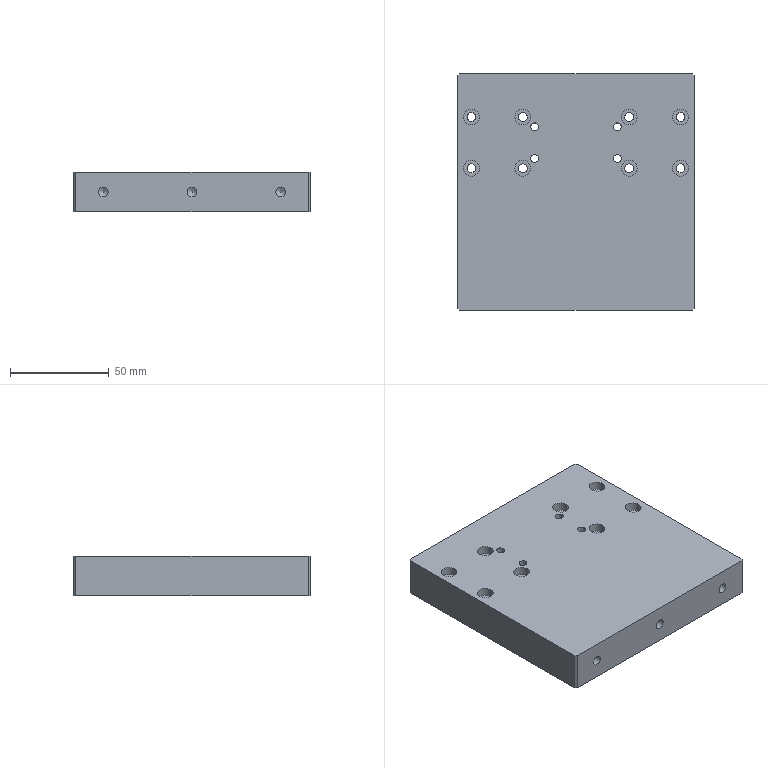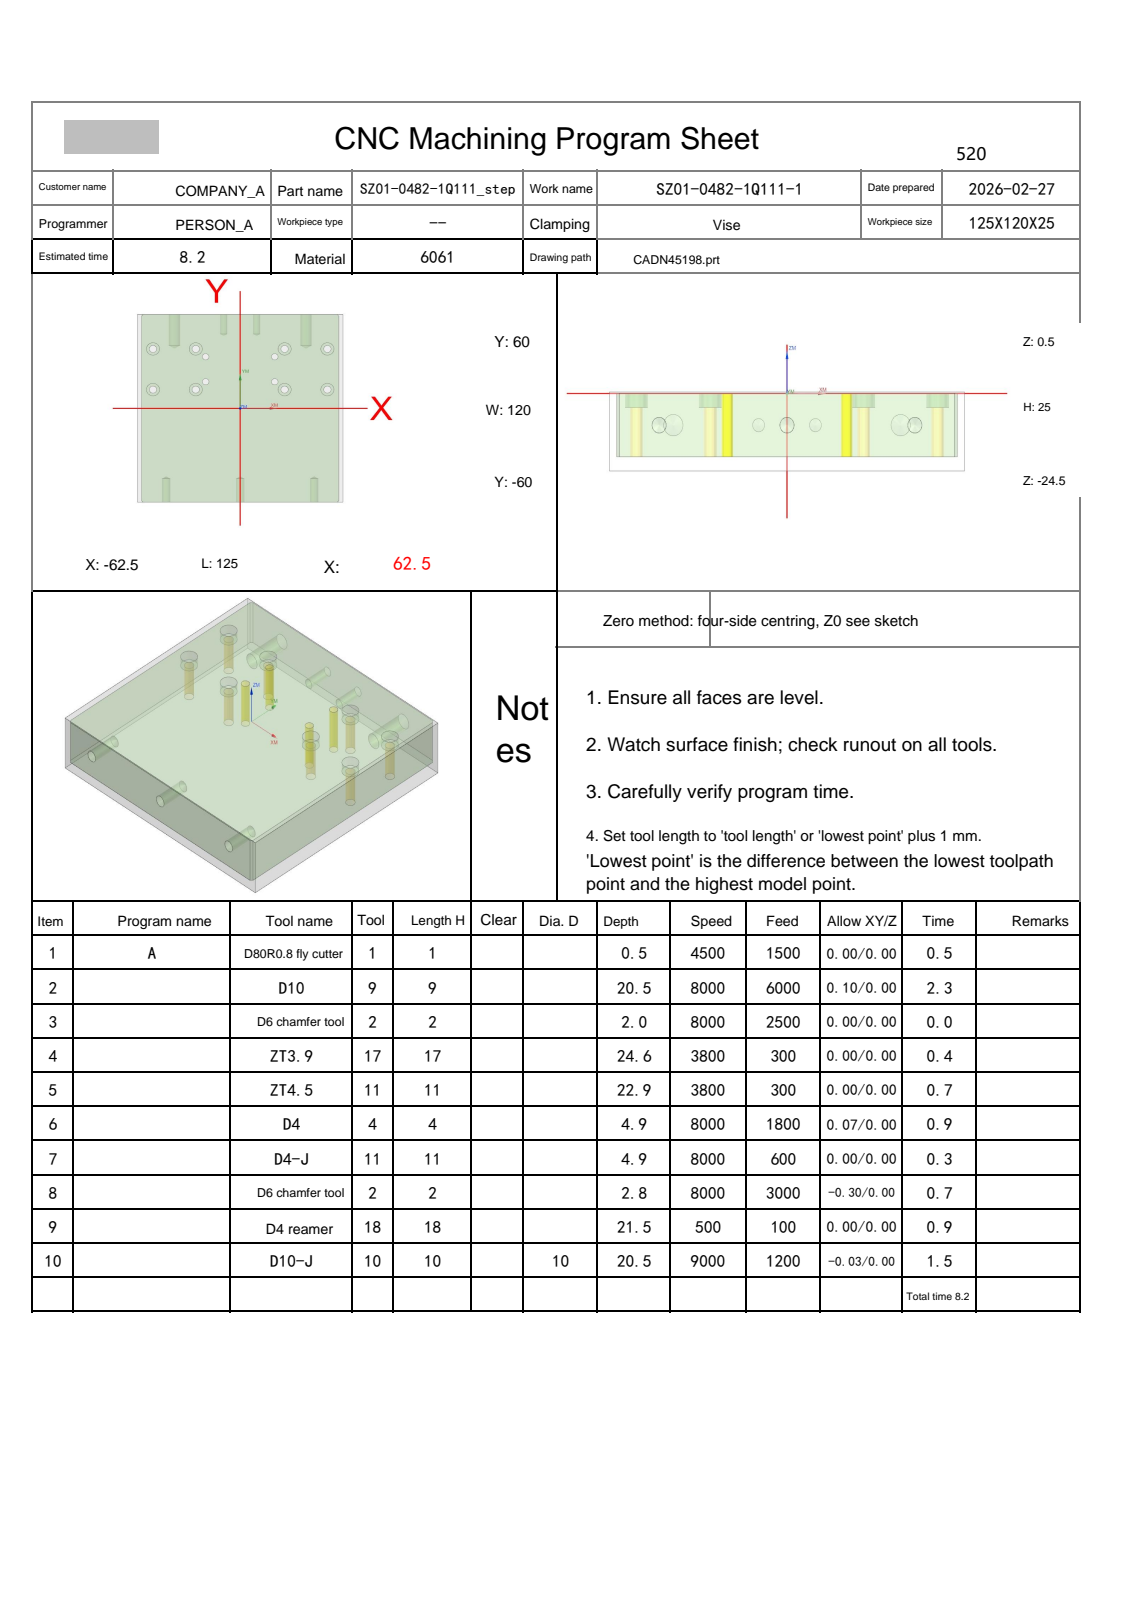NC program | NX | posted by the shop | part box 120 x 120 x 20 mm
Whole program:
%
O0001
(Machine time: 10.07 MIN)
(===Total Tool:8===)
(T1=D80R0.8 fly cutter D=80.  R=0.8  D-  H01 Z=0.    )
(T9=D10     D=10.  R=0.   D-  H09 Z=-20.  )
(T2=D6 chamfer tool   D=6.   R=0.   D-  H02 Z=-2.3  )
(T17=ZT3.9  D=3.9  DR_a=120 D-  H17 Z=-24.13)
(T11=ZT4.5  D=4.5  DR_a=118 D-  H11 Z=-22.35)
(T4=D4      D=4.   R=0.   D-  H04 Z=-4.4  )
(T18=D4 reamer   D=4.   DR_a=180 D-  H18 Z=-21.  )
(T10=D10-J  D=10.  R=0.   D10 H10 Z=-20.  )
G80 G90 G17 G49 G40
G91 G28 Z0
M01
N1 T01 M06
(D80R0.8 fly cutter  D=80. R=0.8 H=01 ce=0.00 di=0.00)
G00 G90 G54 X-105. Y50. M03 S4500
G43 H01 Z50.
M08
Z2.
G01 Z0.0 F1500.
X-100.
X100.
Y0.0
X-100.
Y-50.
X100.
X105.
Z2.
G00 Z50.
G91 G28 Z0.0
M05
M09
G91 G28 Z0.0
M01
N2 T09 M06
(D10  D=10. R=0. H=09 ce=0.10 di=0.00)
G00 G90 G54 X65.1 Y0.0 M03 S8000
G43 H09 Z50.
M08
Z.5
G01 Y-59. Z.409 F6000.
G02 X63.606 Y-62.606 Z.403 I-5.1 J0.0
G01 X62.606 Y-63.606 Z.4
G02 X59. Y-65.1 Z.394 I-3.606 J3.606
G01 X-59. Z.212
G02 X-61.112 Y-64.642 Z.208 I0.0 J5.1
X-62.606 Y-63.606 Z.205 I2.112 J4.642
G01 X-63.606 Y-62.606 Z.203
G02 X-65.1 Y-59. Z.197 I3.606 J3.606
G01 Y59. Z.015
G02 X-63.606 Y62.606 Z.008 I5.1 J0.0
G01 X-62.606 Y63.606 Z.006
G02 X-59. Y65.1 Z0.0 I3.606 J-3.606
G01 X59. Z-.183
G02 X62.606 Y63.606 Z-.189 I0.0 J-5.1
G01 X63.606 Y62.606 Z-.191
G02 X65.1 Y59. Z-.197 I-3.606 J-3.606
G01 Y-59. Z-.38
G02 X63.606 Y-62.606 Z-.386 I-5.1 J0.0
G01 X62.606 Y-63.606 Z-.388
G02 X59. Y-65.1 Z-.394 I-3.606 J3.606
G01 X-59. Z-.577
G02 X-61.112 Y-64.642 Z-.58 I0.0 J5.1
X-62.606 Y-63.606 Z-.583 I2.112 J4.642
G01 X-63.606 Y-62.606 Z-.585
G02 X-65.1 Y-59. Z-.591 I3.606 J3.606
G01 Y59. Z-.774
G02 X-63.606 Y62.606 Z-.78 I5.1 J0.0
G01 X-62.606 Y63.606 Z-.782
G02 X-59. Y65.1 Z-.789 I3.606 J-3.606
G01 X59. Z-.971
G02 X62.606 Y63.606 Z-.977 I0.0 J-5.1
G01 X63.606 Y62.606 Z-.979
G02 X65.1 Y59. Z-.986 I-3.606 J-3.606
G01 Y-59. Z-1.168
G02 X63.606 Y-62.606 Z-1.174 I-5.1 J0.0
G01 X62.606 Y-63.606 Z-1.177
G02 X59. Y-65.1 Z-1.183 I-3.606 J3.606
G01 X-59. Z-1.365
G02 X-61.112 Y-64.642 Z-1.369 I0.0 J5.1
X-62.606 Y-63.606 Z-1.372 I2.112 J4.642
G01 X-63.606 Y-62.606 Z-1.374
G02 X-65.1 Y-59. Z-1.38 I3.606 J3.606
G01 Y59. Z-1.562
G02 X-63.606 Y62.606 Z-1.569 I5.1 J0.0
G01 X-62.606 Y63.606 Z-1.571
G02 X-59. Y65.1 Z-1.577 I3.606 J-3.606
G01 X59. Z-1.76
G02 X62.606 Y63.606 Z-1.766 I0.0 J-5.1
G01 X63.606 Y62.606 Z-1.768
G02 X65.1 Y59. Z-1.774 I-3.606 J-3.606
G01 Y-59. Z-1.957
G02 X63.606 Y-62.606 Z-1.963 I-5.1 J0.0
G01 X62.606 Y-63.606 Z-1.965
G02 X59. Y-65.1 Z-1.971 I-3.606 J3.606
G01 X-59. Z-2.154
G02 X-61.112 Y-64.642 Z-2.157 I0.0 J5.1
X-62.606 Y-63.606 Z-2.16 I2.112 J4.642
G01 X-63.606 Y-62.606 Z-2.162
G02 X-65.1 Y-59. Z-2.168 I3.606 J3.606
G01 Y59. Z-2.351
G02 X-63.606 Y62.606 Z-2.357 I5.1 J0.0
G01 X-62.606 Y63.606 Z-2.359
G02 X-59. Y65.1 Z-2.365 I3.606 J-3.606
G01 X59. Z-2.548
G02 X62.606 Y63.606 Z-2.554 I0.0 J-5.1
G01 X63.606 Y62.606 Z-2.556
G02 X65.1 Y59. Z-2.563 I-3.606 J-3.606
G01 Y-59. Z-2.745
G02 X63.606 Y-62.606 Z-2.751 I-5.1 J0.0
G01 X62.606 Y-63.606 Z-2.753
G02 X59. Y-65.1 Z-2.76 I-3.606 J3.606
G01 X-59. Z-2.942
G02 X-61.112 Y-64.642 Z-2.946 I0.0 J5.1
X-62.606 Y-63.606 Z-2.948 I2.112 J4.642
G01 X-63.606 Y-62.606 Z-2.951
G02 X-65.1 Y-59. Z-2.957 I3.606 J3.606
G01 Y59. Z-3.139
G02 X-63.606 Y62.606 Z-3.146 I5.1 J0.0
G01 X-62.606 Y63.606 Z-3.148
G02 X-59. Y65.1 Z-3.154 I3.606 J-3.606
G01 X59. Z-3.336
G02 X62.606 Y63.606 Z-3.343 I0.0 J-5.1
G01 X63.606 Y62.606 Z-3.345
G02 X65.1 Y59. Z-3.351 I-3.606 J-3.606
G01 Y-59. Z-3.534
G02 X63.606 Y-62.606 Z-3.54 I-5.1 J0.0
G01 X62.606 Y-63.606 Z-3.542
G02 X59. Y-65.1 Z-3.548 I-3.606 J3.606
G01 X-59. Z-3.731
G02 X-61.112 Y-64.642 Z-3.734 I0.0 J5.1
X-62.606 Y-63.606 Z-3.737 I2.112 J4.642
G01 X-63.606 Y-62.606 Z-3.739
G02 X-65.1 Y-59. Z-3.745 I3.606 J3.606
G01 Y59. Z-3.928
G02 X-63.606 Y62.606 Z-3.934 I5.1 J0.0
G01 X-62.606 Y63.606 Z-3.936
G02 X-59. Y65.1 Z-3.942 I3.606 J-3.606
G01 X59. Z-4.125
G02 X62.606 Y63.606 Z-4.131 I0.0 J-5.1
G01 X63.606 Y62.606 Z-4.133
G02 X65.1 Y59. Z-4.14 I-3.606 J-3.606
G01 Y-59. Z-4.322
G02 X63.606 Y-62.606 Z-4.328 I-5.1 J0.0
G01 X62.606 Y-63.606 Z-4.33
G02 X59. Y-65.1 Z-4.337 I-3.606 J3.606
G01 X-59. Z-4.519
G02 X-61.112 Y-64.642 Z-4.523 I0.0 J5.1
X-62.606 Y-63.606 Z-4.525 I2.112 J4.642
G01 X-63.606 Y-62.606 Z-4.528
G02 X-65.1 Y-59. Z-4.534 I3.606 J3.606
G01 Y59. Z-4.716
G02 X-63.606 Y62.606 Z-4.722 I5.1 J0.0
G01 X-62.606 Y63.606 Z-4.725
G02 X-59. Y65.1 Z-4.731 I3.606 J-3.606
G01 X59. Z-4.913
G02 X62.606 Y63.606 Z-4.92 I0.0 J-5.1
G01 X63.606 Y62.606 Z-4.922
G02 X65.1 Y59. Z-4.928 I-3.606 J-3.606
G01 Y-59. Z-5.11
G02 X63.606 Y-62.606 Z-5.117 I-5.1 J0.0
G01 X62.606 Y-63.606 Z-5.119
G02 X59. Y-65.1 Z-5.125 I-3.606 J3.606
G01 X-59. Z-5.308
G02 X-61.112 Y-64.642 Z-5.311 I0.0 J5.1
X-62.606 Y-63.606 Z-5.314 I2.112 J4.642
G01 X-63.606 Y-62.606 Z-5.316
G02 X-65.1 Y-59. Z-5.322 I3.606 J3.606
G01 Y59. Z-5.505
G02 X-63.606 Y62.606 Z-5.511 I5.1 J0.0
G01 X-62.606 Y63.606 Z-5.513
G02 X-59. Y65.1 Z-5.519 I3.606 J-3.606
G01 X59. Z-5.702
G02 X62.606 Y63.606 Z-5.708 I0.0 J-5.1
G01 X63.606 Y62.606 Z-5.71
G02 X65.1 Y59. Z-5.716 I-3.606 J-3.606
G01 Y-59. Z-5.899
G02 X63.606 Y-62.606 Z-5.905 I-5.1 J0.0
G01 X62.606 Y-63.606 Z-5.907
G02 X59. Y-65.1 Z-5.914 I-3.606 J3.606
G01 X-59. Z-6.096
G02 X-61.112 Y-64.642 Z-6.099 I0.0 J5.1
X-62.606 Y-63.606 Z-6.102 I2.112 J4.642
G01 X-63.606 Y-62.606 Z-6.104
G02 X-65.1 Y-59. Z-6.111 I3.606 J3.606
G01 Y59. Z-6.293
G02 X-63.606 Y62.606 Z-6.299 I5.1 J0.0
G01 X-62.606 Y63.606 Z-6.302
G02 X-59. Y65.1 Z-6.308 I3.606 J-3.606
G01 X59. Z-6.49
G02 X62.606 Y63.606 Z-6.497 I0.0 J-5.1
G01 X63.606 Y62.606 Z-6.499
G02 X65.1 Y59. Z-6.505 I-3.606 J-3.606
G01 Y-59. Z-6.687
G02 X63.606 Y-62.606 Z-6.694 I-5.1 J0.0
G01 X62.606 Y-63.606 Z-6.696
G02 X59. Y-65.1 Z-6.702 I-3.606 J3.606
G01 X-59. Z-6.885
G02 X-61.112 Y-64.642 Z-6.888 I0.0 J5.1
X-62.606 Y-63.606 Z-6.891 I2.112 J4.642
G01 X-63.606 Y-62.606 Z-6.893
G02 X-65.1 Y-59. Z-6.899 I3.606 J3.606
G01 Y59. Z-7.082
G02 X-63.606 Y62.606 Z-7.088 I5.1 J0.0
G01 X-62.606 Y63.606 Z-7.09
G02 X-59. Y65.1 Z-7.096 I3.606 J-3.606
G01 X59. Z-7.279
G02 X62.606 Y63.606 Z-7.285 I0.0 J-5.1
G01 X63.606 Y62.606 Z-7.287
G02 X65.1 Y59. Z-7.293 I-3.606 J-3.606
G01 Y-59. Z-7.476
G02 X63.606 Y-62.606 Z-7.482 I-5.1 J0.0
G01 X62.606 Y-63.606 Z-7.484
G02 X59. Y-65.1 Z-7.49 I-3.606 J3.606
G01 X-59. Z-7.673
G02 X-61.112 Y-64.642 Z-7.676 I0.0 J5.1
X-62.606 Y-63.606 Z-7.679 I2.112 J4.642
G01 X-63.606 Y-62.606 Z-7.681
G02 X-65.1 Y-59. Z-7.688 I3.606 J3.606
G01 Y59. Z-7.87
G02 X-63.606 Y62.606 Z-7.876 I5.1 J0.0
G01 X-62.606 Y63.606 Z-7.878
G02 X-59. Y65.1 Z-7.885 I3.606 J-3.606
G01 X59. Z-8.067
G02 X62.606 Y63.606 Z-8.073 I0.0 J-5.1
G01 X63.606 Y62.606 Z-8.076
G02 X65.1 Y59. Z-8.082 I-3.606 J-3.606
G01 Y-59. Z-8.264
G02 X63.606 Y-62.606 Z-8.271 I-5.1 J0.0
G01 X62.606 Y-63.606 Z-8.273
G02 X59. Y-65.1 Z-8.279 I-3.606 J3.606
G01 X-59. Z-8.461
G02 X-61.112 Y-64.642 Z-8.465 I0.0 J5.1
X-62.606 Y-63.606 Z-8.468 I2.112 J4.642
G01 X-63.606 Y-62.606 Z-8.47
G02 X-65.1 Y-59. Z-8.476 I3.606 J3.606
G01 Y59. Z-8.659
G02 X-63.606 Y62.606 Z-8.665 I5.1 J0.0
G01 X-62.606 Y63.606 Z-8.667
G02 X-59. Y65.1 Z-8.673 I3.606 J-3.606
G01 X59. Z-8.856
G02 X62.606 Y63.606 Z-8.862 I0.0 J-5.1
G01 X63.606 Y62.606 Z-8.864
G02 X65.1 Y59. Z-8.87 I-3.606 J-3.606
G01 Y-59. Z-9.053
G02 X63.606 Y-62.606 Z-9.059 I-5.1 J0.0
G01 X62.606 Y-63.606 Z-9.061
G02 X59. Y-65.1 Z-9.067 I-3.606 J3.606
G01 X-59. Z-9.25
G02 X-61.112 Y-64.642 Z-9.253 I0.0 J5.1
X-62.606 Y-63.606 Z-9.256 I2.112 J4.642
G01 X-63.606 Y-62.606 Z-9.258
G02 X-65.1 Y-59. Z-9.265 I3.606 J3.606
G01 Y59. Z-9.447
G02 X-63.606 Y62.606 Z-9.453 I5.1 J0.0
G01 X-62.606 Y63.606 Z-9.455
G02 X-59. Y65.1 Z-9.462 I3.606 J-3.606
G01 X59. Z-9.644
G02 X62.606 Y63.606 Z-9.65 I0.0 J-5.1
G01 X63.606 Y62.606 Z-9.653
G02 X65.1 Y59. Z-9.659 I-3.606 J-3.606
G01 Y-59. Z-9.841
G02 X63.606 Y-62.606 Z-9.847 I-5.1 J0.0
G01 X62.606 Y-63.606 Z-9.85
G02 X59. Y-65.1 Z-9.856 I-3.606 J3.606
G01 X-59. Z-10.038
G02 X-61.112 Y-64.642 Z-10.042 I0.0 J5.1
X-62.606 Y-63.606 Z-10.045 I2.112 J4.642
G01 X-63.606 Y-62.606 Z-10.047
G02 X-65.1 Y-59. Z-10.053 I3.606 J3.606
G01 Y59. Z-10.235
G02 X-63.606 Y62.606 Z-10.242 I5.1 J0.0
G01 X-62.606 Y63.606 Z-10.244
G02 X-59. Y65.1 Z-10.25 I3.606 J-3.606
G01 X59. Z-10.433
G02 X62.606 Y63.606 Z-10.439 I0.0 J-5.1
G01 X63.606 Y62.606 Z-10.441
G02 X65.1 Y59. Z-10.447 I-3.606 J-3.606
G01 Y-59. Z-10.63
G02 X63.606 Y-62.606 Z-10.636 I-5.1 J0.0
G01 X62.606 Y-63.606 Z-10.638
G02 X59. Y-65.1 Z-10.644 I-3.606 J3.606
G01 X-59. Z-10.827
G02 X-61.112 Y-64.642 Z-10.83 I0.0 J5.1
X-62.606 Y-63.606 Z-10.833 I2.112 J4.642
G01 X-63.606 Y-62.606 Z-10.835
G02 X-65.1 Y-59. Z-10.841 I3.606 J3.606
G01 Y59. Z-11.024
G02 X-63.606 Y62.606 Z-11.03 I5.1 J0.0
G01 X-62.606 Y63.606 Z-11.032
G02 X-59. Y65.1 Z-11.039 I3.606 J-3.606
G01 X59. Z-11.221
G02 X62.606 Y63.606 Z-11.227 I0.0 J-5.1
G01 X63.606 Y62.606 Z-11.229
G02 X65.1 Y59. Z-11.236 I-3.606 J-3.606
G01 Y-59. Z-11.418
G02 X63.606 Y-62.606 Z-11.424 I-5.1 J0.0
G01 X62.606 Y-63.606 Z-11.427
G02 X59. Y-65.1 Z-11.433 I-3.606 J3.606
G01 X-59. Z-11.615
G02 X-61.112 Y-64.642 Z-11.619 I0.0 J5.1
X-62.606 Y-63.606 Z-11.622 I2.112 J4.642
G01 X-63.606 Y-62.606 Z-11.624
G02 X-65.1 Y-59. Z-11.63 I3.606 J3.606
G01 Y59. Z-11.812
G02 X-63.606 Y62.606 Z-11.819 I5.1 J0.0
G01 X-62.606 Y63.606 Z-11.821
G02 X-59. Y65.1 Z-11.827 I3.606 J-3.606
G01 X59. Z-12.01
G02 X62.606 Y63.606 Z-12.016 I0.0 J-5.1
G01 X63.606 Y62.606 Z-12.018
G02 X65.1 Y59. Z-12.024 I-3.606 J-3.606
G01 Y-59. Z-12.207
G02 X63.606 Y-62.606 Z-12.213 I-5.1 J0.0
G01 X62.606 Y-63.606 Z-12.215
G02 X59. Y-65.1 Z-12.221 I-3.606 J3.606
G01 X-59. Z-12.404
G02 X-61.112 Y-64.642 Z-12.407 I0.0 J5.1
X-62.606 Y-63.606 Z-12.41 I2.112 J4.642
G01 X-63.606 Y-62.606 Z-12.412
G02 X-65.1 Y-59. Z-12.418 I3.606 J3.606
G01 Y59. Z-12.601
G02 X-63.606 Y62.606 Z-12.607 I5.1 J0.0
G01 X-62.606 Y63.606 Z-12.609
G02 X-59. Y65.1 Z-12.615 I3.606 J-3.606
G01 X59. Z-12.798
G02 X62.606 Y63.606 Z-12.804 I0.0 J-5.1
G01 X63.606 Y62.606 Z-12.806
G02 X65.1 Y59. Z-12.813 I-3.606 J-3.606
G01 Y-59. Z-12.995
G02 X63.606 Y-62.606 Z-13.001 I-5.1 J0.0
G01 X62.606 Y-63.606 Z-13.003
G02 X59. Y-65.1 Z-13.01 I-3.606 J3.606
G01 X-59. Z-13.192
G02 X-61.112 Y-64.642 Z-13.196 I0.0 J5.1
X-62.606 Y-63.606 Z-13.198 I2.112 J4.642
G01 X-63.606 Y-62.606 Z-13.201
G02 X-65.1 Y-59. Z-13.207 I3.606 J3.606
G01 Y59. Z-13.389
G02 X-63.606 Y62.606 Z-13.396 I5.1 J0.0
G01 X-62.606 Y63.606 Z-13.398
G02 X-59. Y65.1 Z-13.404 I3.606 J-3.606
G01 X59. Z-13.586
G02 X62.606 Y63.606 Z-13.593 I0.0 J-5.1
G01 X63.606 Y62.606 Z-13.595
G02 X65.1 Y59. Z-13.601 I-3.606 J-3.606
G01 Y-59. Z-13.784
G02 X63.606 Y-62.606 Z-13.79 I-5.1 J0.0
G01 X62.606 Y-63.606 Z-13.792
G02 X59. Y-65.1 Z-13.798 I-3.606 J3.606
G01 X-59. Z-13.981
G02 X-61.112 Y-64.642 Z-13.984 I0.0 J5.1
X-62.606 Y-63.606 Z-13.987 I2.112 J4.642
G01 X-63.606 Y-62.606 Z-13.989
G02 X-65.1 Y-59. Z-13.995 I3.606 J3.606
G01 Y59. Z-14.178
G02 X-63.606 Y62.606 Z-14.184 I5.1 J0.0
G01 X-62.606 Y63.606 Z-14.186
G02 X-59. Y65.1 Z-14.192 I3.606 J-3.606
G01 X59. Z-14.375
G02 X62.606 Y63.606 Z-14.381 I0.0 J-5.1
G01 X63.606 Y62.606 Z-14.383
G02 X65.1 Y59. Z-14.39 I-3.606 J-3.606
G01 Y-59. Z-14.572
G02 X63.606 Y-62.606 Z-14.578 I-5.1 J0.0
G01 X62.606 Y-63.606 Z-14.58
G02 X59. Y-65.1 Z-14.587 I-3.606 J3.606
G01 X-59. Z-14.769
G02 X-61.112 Y-64.642 Z-14.773 I0.0 J5.1
X-62.606 Y-63.606 Z-14.775 I2.112 J4.642
G01 X-63.606 Y-62.606 Z-14.778
G02 X-65.1 Y-59. Z-14.784 I3.606 J3.606
G01 Y59. Z-14.966
G02 X-63.606 Y62.606 Z-14.972 I5.1 J0.0
G01 X-62.606 Y63.606 Z-14.975
G02 X-59. Y65.1 Z-14.981 I3.606 J-3.606
G01 X59. Z-15.163
G02 X62.606 Y63.606 Z-15.17 I0.0 J-5.1
G01 X63.606 Y62.606 Z-15.172
G02 X65.1 Y59. Z-15.178 I-3.606 J-3.606
G01 Y-59. Z-15.36
G02 X63.606 Y-62.606 Z-15.367 I-5.1 J0.0
G01 X62.606 Y-63.606 Z-15.369
G02 X59. Y-65.1 Z-15.375 I-3.606 J3.606
G01 X-59. Z-15.558
G02 X-61.112 Y-64.642 Z-15.561 I0.0 J5.1
X-62.606 Y-63.606 Z-15.564 I2.112 J4.642
G01 X-63.606 Y-62.606 Z-15.566
G02 X-65.1 Y-59. Z-15.572 I3.606 J3.606
G01 Y59. Z-15.755
G02 X-63.606 Y62.606 Z-15.761 I5.1 J0.0
G01 X-62.606 Y63.606 Z-15.763
G02 X-59. Y65.1 Z-15.769 I3.606 J-3.606
G01 X59. Z-15.952
G02 X62.606 Y63.606 Z-15.958 I0.0 J-5.1
G01 X63.606 Y62.606 Z-15.96
G02 X65.1 Y59. Z-15.966 I-3.606 J-3.606
G01 Y-59. Z-16.149
G02 X63.606 Y-62.606 Z-16.155 I-5.1 J0.0
G01 X62.606 Y-63.606 Z-16.157
G02 X59. Y-65.1 Z-16.164 I-3.606 J3.606
G01 X-59. Z-16.346
G02 X-61.112 Y-64.642 Z-16.349 I0.0 J5.1
X-62.606 Y-63.606 Z-16.352 I2.112 J4.642
G01 X-63.606 Y-62.606 Z-16.354
G02 X-65.1 Y-59. Z-16.361 I3.606 J3.606
G01 Y59. Z-16.543
G02 X-63.606 Y62.606 Z-16.549 I5.1 J0.0
G01 X-62.606 Y63.606 Z-16.552
G02 X-59. Y65.1 Z-16.558 I3.606 J-3.606
G01 X59. Z-16.74
G02 X62.606 Y63.606 Z-16.747 I0.0 J-5.1
G01 X63.606 Y62.606 Z-16.749
G02 X65.1 Y59. Z-16.755 I-3.606 J-3.606
G01 Y-59. Z-16.937
G02 X63.606 Y-62.606 Z-16.944 I-5.1 J0.0
G01 X62.606 Y-63.606 Z-16.946
G02 X59. Y-65.1 Z-16.952 I-3.606 J3.606
G01 X-59. Z-17.135
G02 X-61.112 Y-64.642 Z-17.138 I0.0 J5.1
X-62.606 Y-63.606 Z-17.141 I2.112 J4.642
G01 X-63.606 Y-62.606 Z-17.143
G02 X-65.1 Y-59. Z-17.149 I3.606 J3.606
G01 Y59. Z-17.332
G02 X-63.606 Y62.606 Z-17.338 I5.1 J0.0
G01 X-62.606 Y63.606 Z-17.34
G02 X-59. Y65.1 Z-17.346 I3.606 J-3.606
G01 X59. Z-17.529
G02 X62.606 Y63.606 Z-17.535 I0.0 J-5.1
G01 X63.606 Y62.606 Z-17.537
G02 X65.1 Y59. Z-17.543 I-3.606 J-3.606
G01 Y-59. Z-17.726
G02 X63.606 Y-62.606 Z-17.732 I-5.1 J0.0
G01 X62.606 Y-63.606 Z-17.734
G02 X59. Y-65.1 Z-17.74 I-3.606 J3.606
G01 X-59. Z-17.923
G02 X-61.112 Y-64.642 Z-17.926 I0.0 J5.1
X-62.606 Y-63.606 Z-17.929 I2.112 J4.642
G01 X-63.606 Y-62.606 Z-17.931
G02 X-65.1 Y-59. Z-17.938 I3.606 J3.606
G01 Y59. Z-18.12
G02 X-63.606 Y62.606 Z-18.126 I5.1 J0.0
G01 X-62.606 Y63.606 Z-18.128
G02 X-59. Y65.1 Z-18.135 I3.606 J-3.606
G01 X59. Z-18.317
G02 X62.606 Y63.606 Z-18.323 I0.0 J-5.1
G01 X63.606 Y62.606 Z-18.326
G02 X65.1 Y59. Z-18.332 I-3.606 J-3.606
G01 Y-59. Z-18.514
G02 X63.606 Y-62.606 Z-18.521 I-5.1 J0.0
G01 X62.606 Y-63.606 Z-18.523
G02 X59. Y-65.1 Z-18.529 I-3.606 J3.606
G01 X-59. Z-18.711
G02 X-61.112 Y-64.642 Z-18.715 I0.0 J5.1
X-62.606 Y-63.606 Z-18.718 I2.112 J4.642
G01 X-63.606 Y-62.606 Z-18.72
G02 X-65.1 Y-59. Z-18.726 I3.606 J3.606
G01 Y59. Z-18.909
G02 X-63.606 Y62.606 Z-18.915 I5.1 J0.0
G01 X-62.606 Y63.606 Z-18.917
G02 X-59. Y65.1 Z-18.923 I3.606 J-3.606
G01 X59. Z-19.106
G02 X62.606 Y63.606 Z-19.112 I0.0 J-5.1
G01 X63.606 Y62.606 Z-19.114
G02 X65.1 Y59. Z-19.12 I-3.606 J-3.606
G01 Y-59. Z-19.303
G02 X63.606 Y-62.606 Z-19.309 I-5.1 J0.0
G01 X62.606 Y-63.606 Z-19.311
G02 X59. Y-65.1 Z-19.317 I-3.606 J3.606
G01 X-59. Z-19.5
G02 X-61.112 Y-64.642 Z-19.503 I0.0 J5.1
X-62.606 Y-63.606 Z-19.506 I2.112 J4.642
G01 X-63.606 Y-62.606 Z-19.508
G02 X-65.1 Y-59. Z-19.515 I3.606 J3.606
G01 Y59. Z-19.697
G02 X-63.606 Y62.606 Z-19.703 I5.1 J0.0
G01 X-62.606 Y63.606 Z-19.705
G02 X-59. Y65.1 Z-19.712 I3.606 J-3.606
G01 X59. Z-19.894
G02 X62.606 Y63.606 Z-19.9 I0.0 J-5.1
G01 X63.606 Y62.606 Z-19.903
G02 X65.1 Y59. Z-19.909 I-3.606 J-3.606
G01 Y0.0 Z-20.
Y-59.
G02 X63.606 Y-62.606 I-5.1 J0.0
G01 X62.606 Y-63.606
G02 X59. Y-65.1 I-3.606 J3.606
G01 X-59.
G02 X-62.606 Y-63.606 I0.0 J5.1
G01 X-63.606 Y-62.606
G02 X-65.1 Y-59. I3.606 J3.606
G01 Y59.
G02 X-63.606 Y62.606 I5.1 J0.0
G01 X-62.606 Y63.606
G02 X-59. Y65.1 I3.606 J-3.606
G01 X59.
G02 X62.606 Y63.606 I0.0 J-5.1
G01 X63.606 Y62.606
G02 X65.1 Y59. I-3.606 J-3.606
G01 Y0.0
Y-.5
Z-19.
G00 Z50.
G91 G28 Z0.0
M05
M09
G91 G28 Z0.0
M01
N3 T02 M06
(D6 chamfer tool  D=6. R=0. H=02 ce=0.00 di=0.00)
G00 G90 G54 X-53. Y38. M03 S8000
G43 H02 Z50.
M08
G98 G81 X-53. Y38. Z-1.5 R1. F2500.
Y12.
X-27.
X-21. Y17.
X-27. Y38.
X-21. Y33.
X21.
X27. Y38.
X21. Y17.
X27. Y12.
X53.
Y38.
G80
G00 Z50.
G91 G28 Z0.0
M05
M09
G91 G28 Z0.0
M01
N4 T17 M06
(ZT3.9 D=3.9 DR_a=120 H=17)
G00 G90 G54 X21. Y17. M03 S3800
G43 H17 Z50.
M08
G98 G83 X21. Y17. Z-24.126 R1. F300. Q2.
Y33.
X-21.
Y17.
G80
G00 Z50.
G91 G28 Z0.0
M05
M09
G91 G28 Z0.0
M01
N5 T11 M06
(ZT4.5 D=4.5 DR_a=118 H=11)
G00 G90 G54 X-53. Y38. M03 S3800
G43 H11 Z50.
M08
G98 G83 X-53. Y38. Z-22.352 R1. F300. Q3.
Y12.
X-27.
Y38.
X27.
Y12.
X53.
Y38.
G80
G00 Z50.
G91 G28 Z0.0
M05
M09
G91 G28 Z0.0
M01
N6 T04 M06
(D4  D=4. R=0. H=04 ce=0.07 di=0.00)
G00 G90 G54 X53. Y38. M03 S8000
G43 H04 Z50.
M08
Z.3
G03 X53.965 Y37.035 I.965 J0.0 F1800.
X54.93 Y38. I0.0 J.965
X54.93 Y38. Z-.05 I-1.93 J0.0
X54.93 Y38. Z-.4 I-1.93 J0.0
X54.93 Y38. Z-.75 I-1.93 J0.0
X54.93 Y38. Z-1.1 I-1.93 J0.0
X54.93 Y38. Z-1.45 I-1.93 J0.0
X54.93 Y38. Z-1.8 I-1.93 J0.0
X54.93 Y38. Z-2.15 I-1.93 J0.0
X54.93 Y38. Z-2.5 I-1.93 J0.0
X54.93 Y38. Z-2.85 I-1.93 J0.0
X54.93 Y38. Z-3.2 I-1.93 J0.0
X54.93 Y38. Z-3.55 I-1.93 J0.0
X54.93 Y38. Z-3.9 I-1.93 J0.0
X54.93 Y38. Z-4.25 I-1.93 J0.0
X51.261 Y38.837 Z-4.4 I-1.93 J0.0
X51.07 Y38. I1.739 J-.837
X53. Y36.07 I1.93 J0.0
X54.93 Y38. I0.0 J1.93
X53. Y39.93 I-1.93 J0.0
X51.261 Y38.837 I0.0 J-1.93
X51.166 Y38.419 I.869 J-.419
X52.131 Y37.454 I.965 J0.0
X53. Y38. I0.0 J.965
G00 Z50.
Y12.
Z.3
G03 X53.965 Y11.035 I.965 J0.0
X54.93 Y12. I0.0 J.965
X54.93 Y12. Z-.05 I-1.93 J0.0
X54.93 Y12. Z-.4 I-1.93 J0.0
X54.93 Y12. Z-.75 I-1.93 J0.0
X54.93 Y12. Z-1.1 I-1.93 J0.0
X54.93 Y12. Z-1.45 I-1.93 J0.0
X54.93 Y12. Z-1.8 I-1.93 J0.0
X54.93 Y12. Z-2.15 I-1.93 J0.0
X54.93 Y12. Z-2.5 I-1.93 J0.0
X54.93 Y12. Z-2.85 I-1.93 J0.0
X54.93 Y12. Z-3.2 I-1.93 J0.0
X54.93 Y12. Z-3.55 I-1.93 J0.0
X54.93 Y12. Z-3.9 I-1.93 J0.0
X54.93 Y12. Z-4.25 I-1.93 J0.0
X51.261 Y12.837 Z-4.4 I-1.93 J0.0
X51.07 Y12. I1.739 J-.837
X53. Y10.07 I1.93 J0.0
X54.93 Y12. I0.0 J1.93
X53. Y13.93 I-1.93 J0.0
X51.261 Y12.837 I0.0 J-1.93
X51.166 Y12.419 I.869 J-.419
X52.131 Y11.454 I.965 J0.0
X53. Y12. I0.0 J.965
G00 Z50.
X27.
Z.3
G03 X27.965 Y11.035 I.965 J0.0
X28.93 Y12. I0.0 J.965
X28.93 Y12. Z-.05 I-1.93 J0.0
X28.93 Y12. Z-.4 I-1.93 J0.0
X28.93 Y12. Z-.75 I-1.93 J0.0
X28.93 Y12. Z-1.1 I-1.93 J0.0
X28.93 Y12. Z-1.45 I-1.93 J0.0
X28.93 Y12. Z-1.8 I-1.93 J0.0
X28.93 Y12. Z-2.15 I-1.93 J0.0
X28.93 Y12. Z-2.5 I-1.93 J0.0
X28.93 Y12. Z-2.85 I-1.93 J0.0
X28.93 Y12. Z-3.2 I-1.93 J0.0
X28.93 Y12. Z-3.55 I-1.93 J0.0
X28.93 Y12. Z-3.9 I-1.93 J0.0
X28.93 Y12. Z-4.25 I-1.93 J0.0
X25.261 Y12.837 Z-4.4 I-1.93 J0.0
X25.07 Y12. I1.739 J-.837
X27. Y10.07 I1.93 J0.0
X28.93 Y12. I0.0 J1.93
X27. Y13.93 I-1.93 J0.0
X25.261 Y12.837 I0.0 J-1.93
X25.166 Y12.419 I.869 J-.419
X26.131 Y11.454 I.965 J0.0
X27. Y12. I0.0 J.965
G00 Z50.
Y38.
Z.3
G03 X27.965 Y37.035 I.965 J0.0
X28.93 Y38. I0.0 J.965
X28.93 Y38. Z-.05 I-1.93 J0.0
X28.93 Y38. Z-.4 I-1.93 J0.0
X28.93 Y38. Z-.75 I-1.93 J0.0
X28.93 Y38. Z-1.1 I-1.93 J0.0
X28.93 Y38. Z-1.45 I-1.93 J0.0
X28.93 Y38. Z-1.8 I-1.93 J0.0
X28.93 Y38. Z-2.15 I-1.93 J0.0
X28.93 Y38. Z-2.5 I-1.93 J0.0
X28.93 Y38. Z-2.85 I-1.93 J0.0
X28.93 Y38. Z-3.2 I-1.93 J0.0
X28.93 Y38. Z-3.55 I-1.93 J0.0
X28.93 Y38. Z-3.9 I-1.93 J0.0
X28.93 Y38. Z-4.25 I-1.93 J0.0
X25.261 Y38.837 Z-4.4 I-1.93 J0.0
X25.07 Y38. I1.739 J-.837
X27. Y36.07 I1.93 J0.0
X28.93 Y38. I0.0 J1.93
X27. Y39.93 I-1.93 J0.0
X25.261 Y38.837 I0.0 J-1.93
X25.166 Y38.419 I.869 J-.419
X26.131 Y37.454 I.965 J0.0
X27. Y38. I0.0 J.965
G00 Z50.
X-27.
Z.3
G03 X-26.035 Y37.035 I.965 J0.0
X-25.07 Y38. I0.0 J.965
X-25.07 Y38. Z-.05 I-1.93 J0.0
X-25.07 Y38. Z-.4 I-1.93 J0.0
X-25.07 Y38. Z-.75 I-1.93 J0.0
X-25.07 Y38. Z-1.1 I-1.93 J0.0
X-25.07 Y38. Z-1.45 I-1.93 J0.0
X-25.07 Y38. Z-1.8 I-1.93 J0.0
X-25.07 Y38. Z-2.15 I-1.93 J0.0
X-25.07 Y38. Z-2.5 I-1.93 J0.0
X-25.07 Y38. Z-2.85 I-1.93 J0.0
X-25.07 Y38. Z-3.2 I-1.93 J0.0
X-25.07 Y38. Z-3.55 I-1.93 J0.0
X-25.07 Y38. Z-3.9 I-1.93 J0.0
X-25.07 Y38. Z-4.25 I-1.93 J0.0
X-28.739 Y38.837 Z-4.4 I-1.93 J0.0
X-28.93 Y38. I1.739 J-.837
X-27. Y36.07 I1.93 J0.0
X-25.07 Y38. I0.0 J1.93
X-27. Y39.93 I-1.93 J0.0
X-28.739 Y38.837 I0.0 J-1.93
X-28.834 Y38.419 I.869 J-.419
X-27.869 Y37.454 I.965 J0.0
X-27. Y38. I0.0 J.965
G00 Z50.
Y12.
Z.3
G03 X-26.035 Y11.035 I.965 J0.0
X-25.07 Y12. I0.0 J.965
X-25.07 Y12. Z-.05 I-1.93 J0.0
X-25.07 Y12. Z-.4 I-1.93 J0.0
X-25.07 Y12. Z-.75 I-1.93 J0.0
X-25.07 Y12. Z-1.1 I-1.93 J0.0
X-25.07 Y12. Z-1.45 I-1.93 J0.0
X-25.07 Y12. Z-1.8 I-1.93 J0.0
X-25.07 Y12. Z-2.15 I-1.93 J0.0
X-25.07 Y12. Z-2.5 I-1.93 J0.0
X-25.07 Y12. Z-2.85 I-1.93 J0.0
X-25.07 Y12. Z-3.2 I-1.93 J0.0
X-25.07 Y12. Z-3.55 I-1.93 J0.0
X-25.07 Y12. Z-3.9 I-1.93 J0.0
X-25.07 Y12. Z-4.25 I-1.93 J0.0
X-28.739 Y12.837 Z-4.4 I-1.93 J0.0
X-28.93 Y12. I1.739 J-.837
X-27. Y10.07 I1.93 J0.0
X-25.07 Y12. I0.0 J1.93
X-27. Y13.93 I-1.93 J0.0
X-28.739 Y12.837 I0.0 J-1.93
X-28.834 Y12.419 I.869 J-.419
X-27.869 Y11.454 I.965 J0.0
X-27. Y12. I0.0 J.965
G00 Z50.
X-53.
Z.3
G03 X-52.035 Y11.035 I.965 J0.0
X-51.07 Y12. I0.0 J.965
X-51.07 Y12. Z-.05 I-1.93 J0.0
X-51.07 Y12. Z-.4 I-1.93 J0.0
X-51.07 Y12. Z-.75 I-1.93 J0.0
X-51.07 Y12. Z-1.1 I-1.93 J0.0
X-51.07 Y12. Z-1.45 I-1.93 J0.0
X-51.07 Y12. Z-1.8 I-1.93 J0.0
X-51.07 Y12. Z-2.15 I-1.93 J0.0
X-51.07 Y12. Z-2.5 I-1.93 J0.0
X-51.07 Y12. Z-2.85 I-1.93 J0.0
X-51.07 Y12. Z-3.2 I-1.93 J0.0
X-51.07 Y12. Z-3.55 I-1.93 J0.0
X-51.07 Y12. Z-3.9 I-1.93 J0.0
X-51.07 Y12. Z-4.25 I-1.93 J0.0
X-54.739 Y12.837 Z-4.4 I-1.93 J0.0
X-54.93 Y12. I1.739 J-.837
X-53. Y10.07 I1.93 J0.0
X-51.07 Y12. I0.0 J1.93
X-53. Y13.93 I-1.93 J0.0
X-54.739 Y12.837 I0.0 J-1.93
X-54.834 Y12.419 I.869 J-.419
X-53.869 Y11.454 I.965 J0.0
X-53. Y12. I0.0 J.965
G00 Z50.
Y38.
Z.3
G03 X-52.035 Y37.035 I.965 J0.0
X-51.07 Y38. I0.0 J.965
X-51.07 Y38. Z-.05 I-1.93 J0.0
X-51.07 Y38. Z-.4 I-1.93 J0.0
X-51.07 Y38. Z-.75 I-1.93 J0.0
X-51.07 Y38. Z-1.1 I-1.93 J0.0
X-51.07 Y38. Z-1.45 I-1.93 J0.0
X-51.07 Y38. Z-1.8 I-1.93 J0.0
X-51.07 Y38. Z-2.15 I-1.93 J0.0
X-51.07 Y38. Z-2.5 I-1.93 J0.0
X-51.07 Y38. Z-2.85 I-1.93 J0.0
X-51.07 Y38. Z-3.2 I-1.93 J0.0
X-51.07 Y38. Z-3.55 I-1.93 J0.0
X-51.07 Y38. Z-3.9 I-1.93 J0.0
X-51.07 Y38. Z-4.25 I-1.93 J0.0
X-54.739 Y38.837 Z-4.4 I-1.93 J0.0
X-54.93 Y38. I1.739 J-.837
X-53. Y36.07 I1.93 J0.0
X-51.07 Y38. I0.0 J1.93
X-53. Y39.93 I-1.93 J0.0
X-54.739 Y38.837 I0.0 J-1.93
X-54.834 Y38.419 I.869 J-.419
X-53.869 Y37.454 I.965 J0.0
X-53. Y38. I0.0 J.965
G00 Z50.
G91 G28 Z0.0
M05
M09
G91 G28 Z0.0
M01
N7 T11 M06
(D4-J  D=4. R=0. H=11 ce=0.00 di=0.00)
G00 G90 G54 X53. Y38. M03 S8000
G43 H11 Z50.
M08
Z-4.4
G01 X54.596 Y37.671 F600.
X54.664 Y37.664
G03 X55. Y38. I0.0 J.336
X53. Y40. I-2. J0.0
X51. Y38. I0.0 J-2.
X53. Y36. I2. J0.0
X55. Y38. I0.0 J2.
X54.938 Y38.495 I-2. J0.0
X54.612 Y38.748 I-.325 J-.083
G01 X54.465 Y38.714
X53. Y38.
G00 Z50.
Y12.
Z-4.4
G01 X54.596 Y11.671
X54.664 Y11.664
G03 X55. Y12. I0.0 J.336
X53. Y14. I-2. J0.0
X51. Y12. I0.0 J-2.
X53. Y10. I2. J0.0
X55. Y12. I0.0 J2.
X54.938 Y12.495 I-2. J0.0
X54.612 Y12.748 I-.325 J-.083
G01 X54.465 Y12.714
X53. Y12.
G00 Z50.
X27.
Z-4.4
G01 X28.596 Y11.671
X28.664 Y11.664
G03 X29. Y12. I0.0 J.336
X27. Y14. I-2. J0.0
X25. Y12. I0.0 J-2.
X27. Y10. I2. J0.0
X29. Y12. I0.0 J2.
X28.938 Y12.495 I-2. J0.0
X28.612 Y12.748 I-.325 J-.083
G01 X28.465 Y12.714
X27. Y12.
G00 Z50.
Y38.
Z-4.4
G01 X28.596 Y37.671
X28.664 Y37.664
G03 X29. Y38. I0.0 J.336
X27. Y40. I-2. J0.0
X25. Y38. I0.0 J-2.
X27. Y36. I2. J0.0
X29. Y38. I0.0 J2.
X28.938 Y38.495 I-2. J0.0
X28.612 Y38.748 I-.325 J-.083
G01 X28.465 Y38.714
X27. Y38.
G00 Z50.
X-27.
Z-4.4
G01 X-25.404 Y37.671
X-25.336 Y37.664
G03 X-25. Y38. I0.0 J.336
X-27. Y40. I-2. J0.0
X-29. Y38. I0.0 J-2.
X-27. Y36. I2. J0.0
X-25. Y38. I0.0 J2.
X-25.062 Y38.495 I-2. J0.0
X-25.388 Y38.748 I-.325 J-.083
G01 X-25.535 Y38.714
X-27. Y38.
G00 Z50.
Y12.
Z-4.4
G01 X-25.404 Y11.671
X-25.336 Y11.664
G03 X-25. Y12. I0.0 J.336
X-27. Y14. I-2. J0.0
X-29. Y12. I0.0 J-2.
X-27. Y10. I2. J0.0
X-25. Y12. I0.0 J2.
X-25.062 Y12.495 I-2. J0.0
X-25.388 Y12.748 I-.325 J-.083
G01 X-25.535 Y12.714
X-27. Y12.
G00 Z50.
X-53.
Z-4.4
G01 X-51.404 Y11.671
X-51.336 Y11.664
G03 X-51. Y12. I0.0 J.336
X-53. Y14. I-2. J0.0
X-55. Y12. I0.0 J-2.
X-53. Y10. I2. J0.0
X-51. Y12. I0.0 J2.
X-51.062 Y12.495 I-2. J0.0
X-51.388 Y12.748 I-.325 J-.083
G01 X-51.535 Y12.714
X-53. Y12.
G00 Z50.
Y38.
Z-4.4
G01 X-51.404 Y37.671
X-51.336 Y37.664
G03 X-51. Y38. I0.0 J.336
X-53. Y40. I-2. J0.0
X-55. Y38. I0.0 J-2.
X-53. Y36. I2. J0.0
X-51. Y38. I0.0 J2.
X-51.062 Y38.495 I-2. J0.0
X-51.388 Y38.748 I-.325 J-.083
G01 X-51.535 Y38.714
X-53. Y38.
G00 Z50.
G91 G28 Z0.0
M05
M09
G91 G28 Z0.0
M01
N8 T02 M06
(D6 chamfer tool  D=6. R=0. H=02 ce=0.00 di=0.00)
G00 G90 G54 X.25 Y-62.128 M03 S8000
G43 H02 Z50.
M08
Z2.099
G01 Z-1.5 F3000.
G03 X.33 Y-61.828 I-.52 J.3
X.03 Y-61.308 I-.6 J0.0
G01 X0.0 Y-61.3
X-59.
X-59.254 Y-61.275
X-59.497 Y-61.201
X-59.722 Y-61.081
X-59.919 Y-60.919
X-60.919 Y-59.919
X-61.081 Y-59.722
X-61.201 Y-59.497
X-61.275 Y-59.254
X-61.3 Y-59.
Y59.
X-61.275 Y59.254
X-61.201 Y59.497
X-61.081 Y59.722
X-60.919 Y59.919
X-59.919 Y60.919
X-59.722 Y61.081
X-59.497 Y61.201
X-59.254 Y61.275
X-59. Y61.3
X59.
X59.254 Y61.275
X59.497 Y61.201
X59.722 Y61.081
X59.919 Y60.919
X60.919 Y59.919
X61.081 Y59.722
X61.201 Y59.497
X61.275 Y59.254
X61.3 Y59.
Y-59.
X61.275 Y-59.254
X61.201 Y-59.497
X61.081 Y-59.722
X60.919 Y-59.919
X59.919 Y-60.919
X59.722 Y-61.081
X59.497 Y-61.201
X59.254 Y-61.275
X59. Y-61.3
X0.0
X-.03 Y-61.308
G03 X-.33 Y-61.828 I.3 J-.52
X-.25 Y-62.128 I.6 J0.0
G01 Z2.099
G00 Z50.
G00 G90 X21. Y17. M03 S8000
Z50.
G98 G81 X21. Y17. Z-2.3 R3. F150.
Y33.
X-21.
Y17.
G80
G00 Z50.
G00 G90 X26.388 Y13.147 M03 S8000
Z50.
Z-1.5
G01 Z-2. F600.
X26.2 Y13.5
G03 X24.7 Y12. I0.0 J-1.5
X27. Y9.7 I2.3 J0.0
X29.3 Y12. I0.0 J2.3
X27. Y14.3 I-2.3 J0.0
X24.7 Y12. I0.0 J-2.3
X26.2 Y10.5 I1.5 J0.0
G01 X26.388 Y10.853
Z-1.5
G00 Z50.
X52.388 Y13.147
Z-1.5
G01 Z-2.
X52.2 Y13.5
G03 X50.7 Y12. I0.0 J-1.5
X53. Y9.7 I2.3 J0.0
X55.3 Y12. I0.0 J2.3
X53. Y14.3 I-2.3 J0.0
X50.7 Y12. I0.0 J-2.3
X52.2 Y10.5 I1.5 J0.0
G01 X52.388 Y10.853
Z-1.5
G00 Z50.
Y39.147
Z-1.5
G01 Z-2.
X52.2 Y39.5
G03 X50.7 Y38. I0.0 J-1.5
X53. Y35.7 I2.3 J0.0
X55.3 Y38. I0.0 J2.3
X53. Y40.3 I-2.3 J0.0
X50.7 Y38. I0.0 J-2.3
X52.2 Y36.5 I1.5 J0.0
G01 X52.388 Y36.853
Z-1.5
G00 Z50.
X26.388 Y39.147
Z-1.5
G01 Z-2.
X26.2 Y39.5
G03 X24.7 Y38. I0.0 J-1.5
X27. Y35.7 I2.3 J0.0
X29.3 Y38. I0.0 J2.3
X27. Y40.3 I-2.3 J0.0
X24.7 Y38. I0.0 J-2.3
X26.2 Y36.5 I1.5 J0.0
G01 X26.388 Y36.853
Z-1.5
G00 Z50.
X-27.612 Y39.147
Z-1.5
G01 Z-2.
X-27.8 Y39.5
G03 X-29.3 Y38. I0.0 J-1.5
X-27. Y35.7 I2.3 J0.0
X-24.7 Y38. I0.0 J2.3
X-27. Y40.3 I-2.3 J0.0
X-29.3 Y38. I0.0 J-2.3
X-27.8 Y36.5 I1.5 J0.0
G01 X-27.612 Y36.853
Z-1.5
G00 Z50.
X-53.612 Y39.147
Z-1.5
G01 Z-2.
X-53.8 Y39.5
G03 X-55.3 Y38. I0.0 J-1.5
X-53. Y35.7 I2.3 J0.0
X-50.7 Y38. I0.0 J2.3
X-53. Y40.3 I-2.3 J0.0
X-55.3 Y38. I0.0 J-2.3
X-53.8 Y36.5 I1.5 J0.0
G01 X-53.612 Y36.853
Z-1.5
G00 Z50.
Y13.147
Z-1.5
G01 Z-2.
X-53.8 Y13.5
G03 X-55.3 Y12. I0.0 J-1.5
X-53. Y9.7 I2.3 J0.0
X-50.7 Y12. I0.0 J2.3
X-53. Y14.3 I-2.3 J0.0
X-55.3 Y12. I0.0 J-2.3
X-53.8 Y10.5 I1.5 J0.0
G01 X-53.612 Y10.853
Z-1.5
G00 Z50.
X-27.612 Y13.147
Z-1.5
G01 Z-2.
X-27.8 Y13.5
G03 X-29.3 Y12. I0.0 J-1.5
X-27. Y9.7 I2.3 J0.0
X-24.7 Y12. I0.0 J2.3
X-27. Y14.3 I-2.3 J0.0
X-29.3 Y12. I0.0 J-2.3
X-27.8 Y10.5 I1.5 J0.0
G01 X-27.612 Y10.853
Z-1.5
G00 Z50.
G91 G28 Z0.0
M05
M09
G91 G28 Z0.0
M01
N9 T18 M06
(D4 reamer D=4. DR_a=180 H=18)
G00 G90 G54 X21. Y17. M03 S500
G43 H18 Z50.
M08
G98 G85 X21. Y17. Z-21. R1. F100.
Y33.
X-21.
Y17.
G80
G00 Z50.
G91 G28 Z0.0
M05
M09
G91 G28 Z0.0
M01
N10 T10 M06
(D10-J  D=10. R=0. H=10 ce=0.00 di=0.00)
G00 G90 G54 X-66.116 Y-60.013 M03 S9000
G43 H10 Z50.
M08
Z-9.5
G01 Z-10. F1200.
G41 D10
X-65.917 Y-59.997
G03 X-65. Y-59. I-.083 J.997
G01 Y59.
G02 X-63.536 Y62.536 I5. J0.0
G01 X-62.536 Y63.536
G02 X-59. Y65. I3.536 J-3.536
G01 X59.
G02 X62.536 Y63.536 I0.0 J-5.
G01 X63.536 Y62.536
G02 X65. Y59. I-3.536 J-3.536
G01 Y-59.
G02 X63.536 Y-62.536 I-5. J0.0
G01 X62.536 Y-63.536
G02 X59. Y-65. I-3.536 J3.536
G01 X-59.
G02 X-62.536 Y-63.536 I0.0 J5.
G01 X-63.536 Y-62.536
G02 X-65. Y-59. I3.536 J3.536
G01 Y-58.5
G03 X-66. Y-57.5 I-1. J0.0
G01 G40 X-66.2
Z-9.5
G00 Z50.
X-66.116 Y-60.013
Z-19.5
G01 Z-20.
G41 D10
X-65.917 Y-59.997
G03 X-65. Y-59. I-.083 J.997
G01 Y59.
G02 X-63.536 Y62.536 I5. J0.0
G01 X-62.536 Y63.536
G02 X-59. Y65. I3.536 J-3.536
G01 X59.
G02 X62.536 Y63.536 I0.0 J-5.
G01 X63.536 Y62.536
G02 X65. Y59. I-3.536 J-3.536
G01 Y-59.
G02 X63.536 Y-62.536 I-5. J0.0
G01 X62.536 Y-63.536
G02 X59. Y-65. I-3.536 J3.536
G01 X-59.
G02 X-62.536 Y-63.536 I0.0 J5.
G01 X-63.536 Y-62.536
G02 X-65. Y-59. I3.536 J3.536
G01 Y-58.5
G03 X-66. Y-57.5 I-1. J0.0
G01 G40 X-66.2
Z-19.5
G00 Z50.
G00 G90 X65.5 Y-66.675 M03 S8000
Z10.5
Z-8.5
G01 Z-10. F1000.
G41 D10
Y-66.475
G03 X64. Y-64.975 I-1.5 J0.0
G01 X-64.
G03 X-65.5 Y-66.475 I0.0 J-1.5
G01 G40 Y-66.675
Z-8.5
G00 X65.5
Z-18.5
G01 Z-20.
G41 D10
Y-66.475
G03 X64. Y-64.975 I-1.5 J0.0
G01 X-64.
G03 X-65.5 Y-66.475 I0.0 J-1.5
G01 G40 Y-66.675
Z-18.5
G00 Z10.5
Y66.675
Z-8.5
G01 Z-10.
G41 D10
Y66.475
G03 X-64. Y64.975 I1.5 J0.0
G01 X64.
G03 X65.5 Y66.475 I0.0 J1.5
G01 G40 Y66.675
Z-8.5
G00 X-65.5
Z-18.5
G01 Z-20.
G41 D10
Y66.475
G03 X-64. Y64.975 I1.5 J0.0
G01 X64.
G03 X65.5 Y66.475 I0.0 J1.5
G01 G40 Y66.675
Z-18.5
G00 Z10.5
M05
M09
G91 G28 Z0.0
G91 G28 Y0.0
M30
%